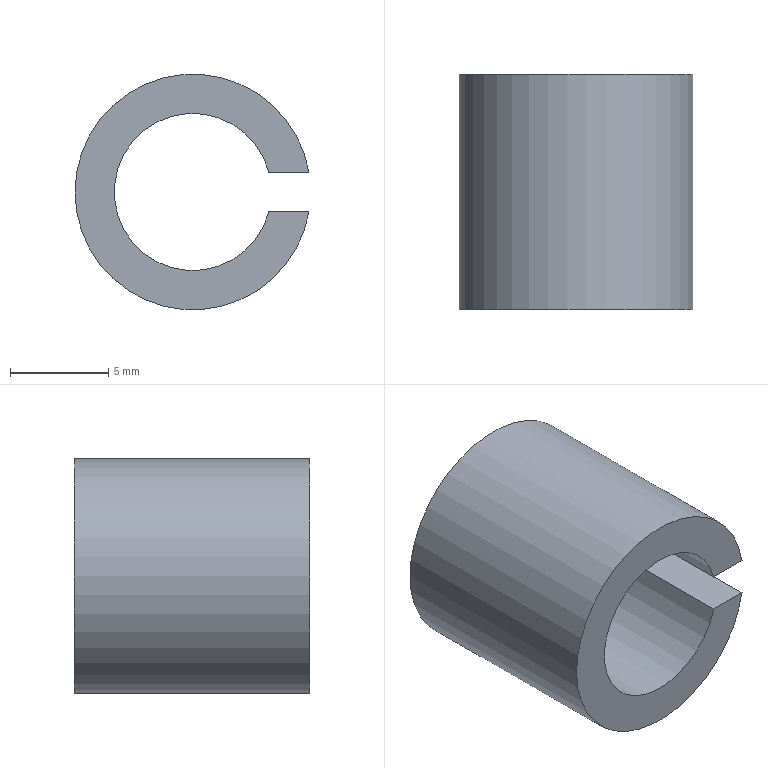Part | NX | features DATUM_CSYS 3, EXTRUDE 2, SKETCH 2 | 1 solid | 6 faces | box 11.916 x 12 x 12 mm | volume 705.642 mm3 | plane 4 | cylinder 2 | commonest cylinder face diameters 8 x1 12 x1
STEP:
#1=CARTESIAN_POINT('',(5.916,-6.,1.));
#2=VERTEX_POINT('',#1);
#3=CARTESIAN_POINT('',(5.916,-6.,-1.));
#4=VERTEX_POINT('',#3);
#5=CARTESIAN_POINT('',(0.,-6.,0.));
#6=DIRECTION('',(0.,-1.,0.));
#7=DIRECTION('',(1.,0.,0.));
#8=AXIS2_PLACEMENT_3D('',#5,#6,#7);
#9=CIRCLE('',#8,6.);
#10=EDGE_CURVE('',#2,#4,#9,.T.);
#11=ORIENTED_EDGE('',*,*,#10,.F.);
#12=CARTESIAN_POINT('',(5.916,6.,1.));
#13=VERTEX_POINT('',#12);
#14=CARTESIAN_POINT('',(5.916,-6.,1.));
#15=DIRECTION('',(0.,1.,0.));
#16=VECTOR('',#15,1000.);
#17=LINE('',#14,#16);
#18=EDGE_CURVE('',#2,#13,#17,.T.);
#19=ORIENTED_EDGE('',*,*,#18,.T.);
#20=CARTESIAN_POINT('',(5.916,6.,-1.));
#21=VERTEX_POINT('',#20);
#22=CARTESIAN_POINT('',(0.,6.,0.));
#23=DIRECTION('',(0.,-1.,0.));
#24=DIRECTION('',(1.,0.,0.));
#25=AXIS2_PLACEMENT_3D('',#22,#23,#24);
#26=CIRCLE('',#25,6.);
#27=EDGE_CURVE('',#13,#21,#26,.T.);
#28=ORIENTED_EDGE('',*,*,#27,.T.);
#29=CARTESIAN_POINT('',(5.916,-6.,-1.));
#30=DIRECTION('',(0.,1.,0.));
#31=VECTOR('',#30,1000.);
#32=LINE('',#29,#31);
#33=EDGE_CURVE('',#21,#4,#32,.F.);
#34=ORIENTED_EDGE('',*,*,#33,.T.);
#35=EDGE_LOOP('',(#11,#19,#28,#34));
#36=FACE_BOUND('',#35,.T.);
#37=CARTESIAN_POINT('',(0.,-6.,0.));
#38=DIRECTION('',(0.,1.,0.));
#39=DIRECTION('',(0.,0.,1.));
#40=AXIS2_PLACEMENT_3D('',#37,#38,#39);
#41=CYLINDRICAL_SURFACE('',#40,6.);
#42=ADVANCED_FACE('',(#36),#41,.T.);
#43=CARTESIAN_POINT('',(3.873,-6.,1.));
#44=VERTEX_POINT('',#43);
#45=CARTESIAN_POINT('',(3.873,6.,1.));
#46=VERTEX_POINT('',#45);
#47=CARTESIAN_POINT('',(3.873,-6.,1.));
#48=DIRECTION('',(0.,1.,0.));
#49=VECTOR('',#48,1000.);
#50=LINE('',#47,#49);
#51=EDGE_CURVE('',#44,#46,#50,.T.);
#52=ORIENTED_EDGE('',*,*,#51,.F.);
#53=CARTESIAN_POINT('',(3.873,-6.,-1.));
#54=VERTEX_POINT('',#53);
#55=CARTESIAN_POINT('',(0.,-6.,0.));
#56=DIRECTION('',(0.,-1.,0.));
#57=DIRECTION('',(1.,0.,0.));
#58=AXIS2_PLACEMENT_3D('',#55,#56,#57);
#59=CIRCLE('',#58,4.);
#60=EDGE_CURVE('',#44,#54,#59,.T.);
#61=ORIENTED_EDGE('',*,*,#60,.T.);
#62=CARTESIAN_POINT('',(3.873,6.,-1.));
#63=VERTEX_POINT('',#62);
#64=CARTESIAN_POINT('',(3.873,-6.,-1.));
#65=DIRECTION('',(0.,1.,0.));
#66=VECTOR('',#65,1000.);
#67=LINE('',#64,#66);
#68=EDGE_CURVE('',#63,#54,#67,.F.);
#69=ORIENTED_EDGE('',*,*,#68,.F.);
#70=CARTESIAN_POINT('',(0.,6.,0.));
#71=DIRECTION('',(0.,-1.,0.));
#72=DIRECTION('',(1.,0.,0.));
#73=AXIS2_PLACEMENT_3D('',#70,#71,#72);
#74=CIRCLE('',#73,4.);
#75=EDGE_CURVE('',#46,#63,#74,.T.);
#76=ORIENTED_EDGE('',*,*,#75,.F.);
#77=EDGE_LOOP('',(#52,#61,#69,#76));
#78=FACE_BOUND('',#77,.T.);
#79=CARTESIAN_POINT('',(0.,-6.,0.));
#80=DIRECTION('',(0.,1.,0.));
#81=DIRECTION('',(0.,0.,1.));
#82=AXIS2_PLACEMENT_3D('',#79,#80,#81);
#83=CYLINDRICAL_SURFACE('',#82,4.);
#84=ADVANCED_FACE('',(#78),#83,.F.);
#85=CARTESIAN_POINT('',(7.1,-6.,1.));
#86=DIRECTION('',(-1.,0.,0.));
#87=VECTOR('',#86,1000.);
#88=LINE('',#85,#87);
#89=EDGE_CURVE('',#2,#44,#88,.T.);
#90=ORIENTED_EDGE('',*,*,#89,.F.);
#91=ORIENTED_EDGE('',*,*,#10,.T.);
#92=CARTESIAN_POINT('',(3.45,-6.,-1.));
#93=DIRECTION('',(1.,0.,0.));
#94=VECTOR('',#93,1000.);
#95=LINE('',#92,#94);
#96=EDGE_CURVE('',#54,#4,#95,.T.);
#97=ORIENTED_EDGE('',*,*,#96,.F.);
#98=ORIENTED_EDGE('',*,*,#60,.F.);
#99=EDGE_LOOP('',(#90,#91,#97,#98));
#100=FACE_BOUND('',#99,.T.);
#101=CARTESIAN_POINT('',(0.,-6.,0.));
#102=DIRECTION('',(0.,-1.,0.));
#103=DIRECTION('',(0.,0.,-1.));
#104=AXIS2_PLACEMENT_3D('',#101,#102,#103);
#105=PLANE('',#104);
#106=ADVANCED_FACE('',(#100),#105,.T.);
#107=ORIENTED_EDGE('',*,*,#27,.F.);
#108=CARTESIAN_POINT('',(0.,6.,1.));
#109=DIRECTION('',(-1.,0.,0.));
#110=VECTOR('',#109,1000.);
#111=LINE('',#108,#110);
#112=EDGE_CURVE('',#13,#46,#111,.T.);
#113=ORIENTED_EDGE('',*,*,#112,.T.);
#114=ORIENTED_EDGE('',*,*,#75,.T.);
#115=CARTESIAN_POINT('',(0.,6.,-1.));
#116=DIRECTION('',(1.,0.,0.));
#117=VECTOR('',#116,1000.);
#118=LINE('',#115,#117);
#119=EDGE_CURVE('',#63,#21,#118,.T.);
#120=ORIENTED_EDGE('',*,*,#119,.T.);
#121=EDGE_LOOP('',(#107,#113,#114,#120));
#122=FACE_BOUND('',#121,.T.);
#123=CARTESIAN_POINT('',(0.,6.,0.));
#124=DIRECTION('',(0.,-1.,0.));
#125=DIRECTION('',(0.,0.,-1.));
#126=AXIS2_PLACEMENT_3D('',#123,#124,#125);
#127=PLANE('',#126);
#128=ADVANCED_FACE('',(#122),#127,.F.);
#129=ORIENTED_EDGE('',*,*,#119,.F.);
#130=ORIENTED_EDGE('',*,*,#68,.T.);
#131=ORIENTED_EDGE('',*,*,#96,.T.);
#132=ORIENTED_EDGE('',*,*,#33,.F.);
#133=EDGE_LOOP('',(#129,#130,#131,#132));
#134=FACE_BOUND('',#133,.T.);
#135=CARTESIAN_POINT('',(3.45,10.,-1.));
#136=DIRECTION('',(0.,0.,-1.));
#137=DIRECTION('',(-1.,0.,0.));
#138=AXIS2_PLACEMENT_3D('',#135,#136,#137);
#139=PLANE('',#138);
#140=ADVANCED_FACE('',(#134),#139,.F.);
#141=ORIENTED_EDGE('',*,*,#89,.T.);
#142=ORIENTED_EDGE('',*,*,#51,.T.);
#143=ORIENTED_EDGE('',*,*,#112,.F.);
#144=ORIENTED_EDGE('',*,*,#18,.F.);
#145=EDGE_LOOP('',(#141,#142,#143,#144));
#146=FACE_BOUND('',#145,.T.);
#147=CARTESIAN_POINT('',(7.1,10.,1.));
#148=DIRECTION('',(0.,0.,1.));
#149=DIRECTION('',(1.,0.,0.));
#150=AXIS2_PLACEMENT_3D('',#147,#148,#149);
#151=PLANE('',#150);
#152=ADVANCED_FACE('',(#146),#151,.F.);
#153=CLOSED_SHELL('',(#42,#84,#106,#128,#140,#152));
#154=MANIFOLD_SOLID_BREP('',#153);
#155=(LENGTH_UNIT()NAMED_UNIT(*)SI_UNIT(.MILLI.,.METRE.));
#156=UNCERTAINTY_MEASURE_WITH_UNIT(LENGTH_MEASURE(0.00001),#155,'','');
#157=(NAMED_UNIT(*)PLANE_ANGLE_UNIT()SI_UNIT($,.RADIAN.));
#158=(NAMED_UNIT(*)SI_UNIT($,.STERADIAN.)SOLID_ANGLE_UNIT());
#159=(GEOMETRIC_REPRESENTATION_CONTEXT(3)GLOBAL_UNCERTAINTY_ASSIGNED_CONTEXT((#156))GLOBAL_UNIT_ASSIGNED_CONTEXT((#155,#157,#158))REPRESENTATION_CONTEXT('',''));
#160=ADVANCED_BREP_SHAPE_REPRESENTATION('',(#154),#159);